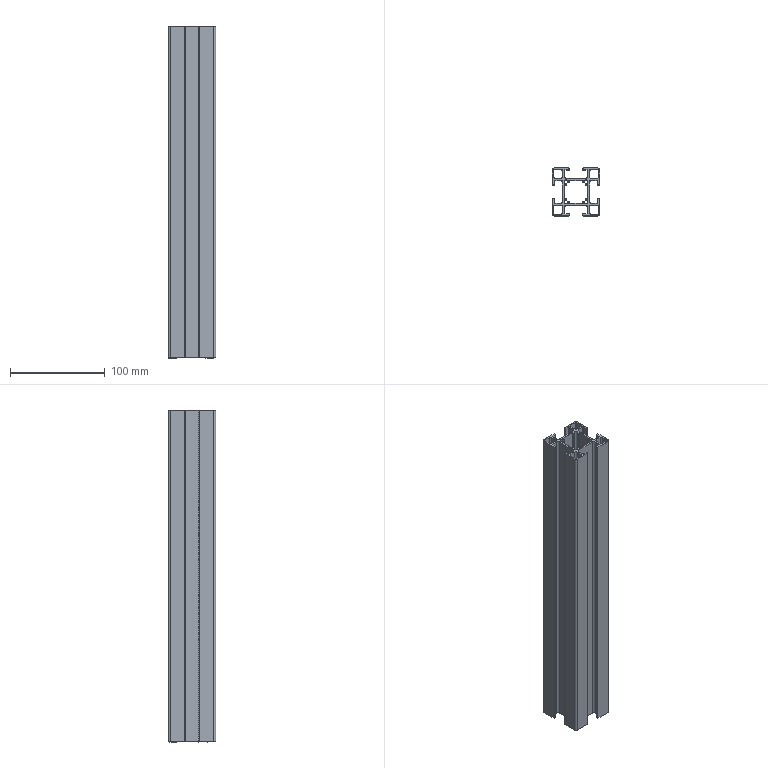Part | STEP file | 46A-00006CC11-350mm | 1 solid | 142 faces | box 50 x 50 x 350 mm | volume 205622 mm3 | cylinder 84 | plane 58 | commonest cylinder face diameters 1 x24 4 x24 1.5 x16 3.7 x8 6.7 x8 2 x4